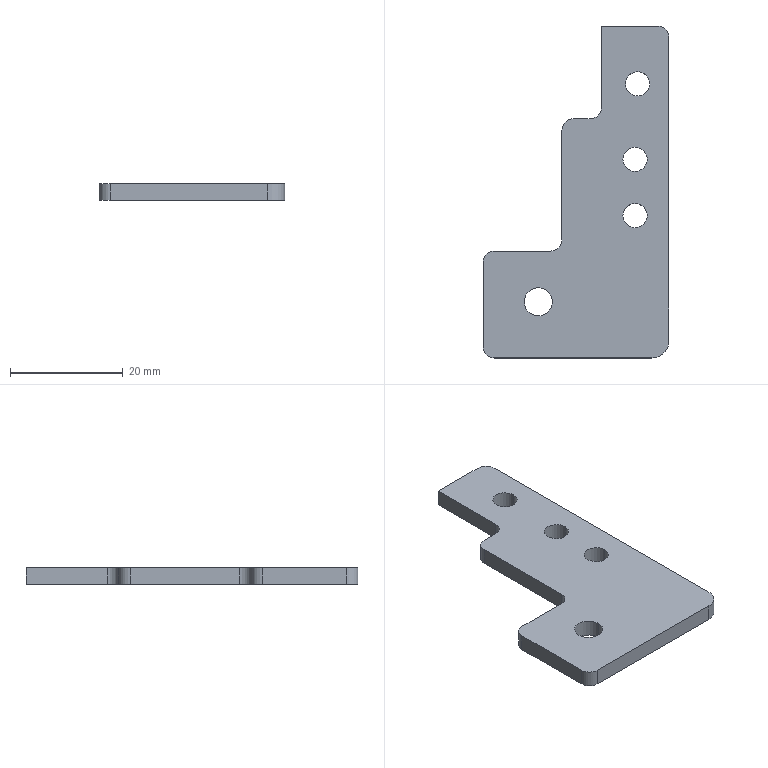Part | SolidWorks | features Cut 4, ICE 4, Fillet 3, MoveFace 2, Extrusion 1, HoleWzd 1 | 1 solid | 25 faces | box 33 x 59 x 3 mm | volume 3614 mm3 | cylinder 15 | plane 10 | commonest cylinder face diameters 4 x6 4.3 x6 5 x2 6 x1
STEP:
#1=CARTESIAN_POINT('',(8.8,19.2,3.));
#2=VERTEX_POINT('',#1);
#3=CARTESIAN_POINT('',(13.1,19.2,3.));
#4=VERTEX_POINT('',#3);
#5=CARTESIAN_POINT('',(10.95,19.2,3.));
#6=DIRECTION('',(0.,0.,1.));
#7=DIRECTION('',(1.,0.,0.));
#8=AXIS2_PLACEMENT_3D('',#5,#6,#7);
#9=CIRCLE('',#8,2.15);
#10=EDGE_CURVE('',#2,#4,#9,.T.);
#11=ORIENTED_EDGE('',*,*,#10,.T.);
#12=CARTESIAN_POINT('',(13.1,19.2,0.));
#13=VERTEX_POINT('',#12);
#14=CARTESIAN_POINT('',(13.1,19.2,0.));
#15=DIRECTION('',(0.,0.,-1.));
#16=VECTOR('',#15,1000.);
#17=LINE('',#14,#16);
#18=EDGE_CURVE('',#4,#13,#17,.T.);
#19=ORIENTED_EDGE('',*,*,#18,.T.);
#20=CARTESIAN_POINT('',(8.8,19.2,0.));
#21=VERTEX_POINT('',#20);
#22=CARTESIAN_POINT('',(10.95,19.2,0.));
#23=DIRECTION('',(0.,0.,-1.));
#24=DIRECTION('',(-1.,0.,0.));
#25=AXIS2_PLACEMENT_3D('',#22,#23,#24);
#26=CIRCLE('',#25,2.15);
#27=EDGE_CURVE('',#13,#21,#26,.T.);
#28=ORIENTED_EDGE('',*,*,#27,.T.);
#29=CARTESIAN_POINT('',(8.8,19.2,0.));
#30=DIRECTION('',(0.,0.,-1.));
#31=VECTOR('',#30,1000.);
#32=LINE('',#29,#31);
#33=EDGE_CURVE('',#2,#21,#32,.T.);
#34=ORIENTED_EDGE('',*,*,#33,.F.);
#35=EDGE_LOOP('',(#11,#19,#28,#34));
#36=FACE_OUTER_BOUND('',#35,.T.);
#37=CARTESIAN_POINT('',(10.95,19.2,0.));
#38=DIRECTION('',(0.,0.,-1.));
#39=DIRECTION('',(-1.,0.,0.));
#40=AXIS2_PLACEMENT_3D('',#37,#38,#39);
#41=CYLINDRICAL_SURFACE('',#40,2.15);
#42=ADVANCED_FACE('',(#36),#41,.F.);
#43=CARTESIAN_POINT('',(-9.2,-19.5,3.));
#44=VERTEX_POINT('',#43);
#45=CARTESIAN_POINT('',(-4.2,-19.5,3.));
#46=VERTEX_POINT('',#45);
#47=CARTESIAN_POINT('',(-6.7,-19.5,3.));
#48=DIRECTION('',(0.,0.,1.));
#49=DIRECTION('',(1.,0.,0.));
#50=AXIS2_PLACEMENT_3D('',#47,#48,#49);
#51=CIRCLE('',#50,2.5);
#52=EDGE_CURVE('',#44,#46,#51,.T.);
#53=ORIENTED_EDGE('',*,*,#52,.T.);
#54=CARTESIAN_POINT('',(-4.2,-19.5,0.));
#55=VERTEX_POINT('',#54);
#56=CARTESIAN_POINT('',(-4.2,-19.5,10.));
#57=DIRECTION('',(0.,0.,-1.));
#58=VECTOR('',#57,1000.);
#59=LINE('',#56,#58);
#60=EDGE_CURVE('',#46,#55,#59,.T.);
#61=ORIENTED_EDGE('',*,*,#60,.T.);
#62=CARTESIAN_POINT('',(-9.2,-19.5,0.));
#63=VERTEX_POINT('',#62);
#64=CARTESIAN_POINT('',(-6.7,-19.5,0.));
#65=DIRECTION('',(0.,0.,-1.));
#66=DIRECTION('',(-1.,0.,0.));
#67=AXIS2_PLACEMENT_3D('',#64,#65,#66);
#68=CIRCLE('',#67,2.5);
#69=EDGE_CURVE('',#55,#63,#68,.T.);
#70=ORIENTED_EDGE('',*,*,#69,.T.);
#71=CARTESIAN_POINT('',(-9.2,-19.5,10.));
#72=DIRECTION('',(0.,0.,-1.));
#73=VECTOR('',#72,1000.);
#74=LINE('',#71,#73);
#75=EDGE_CURVE('',#44,#63,#74,.T.);
#76=ORIENTED_EDGE('',*,*,#75,.F.);
#77=EDGE_LOOP('',(#53,#61,#70,#76));
#78=FACE_OUTER_BOUND('',#77,.T.);
#79=CARTESIAN_POINT('',(-6.7,-19.5,10.));
#80=DIRECTION('',(0.,0.,-1.));
#81=DIRECTION('',(-1.,0.,0.));
#82=AXIS2_PLACEMENT_3D('',#79,#80,#81);
#83=CYLINDRICAL_SURFACE('',#82,2.5);
#84=ADVANCED_FACE('',(#78),#83,.F.);
#85=CARTESIAN_POINT('',(8.35,5.8,3.));
#86=VERTEX_POINT('',#85);
#87=CARTESIAN_POINT('',(12.65,5.8,3.));
#88=VERTEX_POINT('',#87);
#89=CARTESIAN_POINT('',(10.5,5.8,3.));
#90=DIRECTION('',(0.,0.,1.));
#91=DIRECTION('',(1.,0.,0.));
#92=AXIS2_PLACEMENT_3D('',#89,#90,#91);
#93=CIRCLE('',#92,2.15);
#94=EDGE_CURVE('',#86,#88,#93,.T.);
#95=ORIENTED_EDGE('',*,*,#94,.T.);
#96=CARTESIAN_POINT('',(12.65,5.8,0.));
#97=VERTEX_POINT('',#96);
#98=CARTESIAN_POINT('',(12.65,5.8,21.));
#99=DIRECTION('',(0.,0.,-1.));
#100=VECTOR('',#99,1000.);
#101=LINE('',#98,#100);
#102=EDGE_CURVE('',#88,#97,#101,.T.);
#103=ORIENTED_EDGE('',*,*,#102,.T.);
#104=CARTESIAN_POINT('',(8.35,5.8,0.));
#105=VERTEX_POINT('',#104);
#106=CARTESIAN_POINT('',(10.5,5.8,0.));
#107=DIRECTION('',(0.,0.,-1.));
#108=DIRECTION('',(-1.,0.,0.));
#109=AXIS2_PLACEMENT_3D('',#106,#107,#108);
#110=CIRCLE('',#109,2.15);
#111=EDGE_CURVE('',#97,#105,#110,.T.);
#112=ORIENTED_EDGE('',*,*,#111,.T.);
#113=CARTESIAN_POINT('',(8.35,5.8,21.));
#114=DIRECTION('',(0.,0.,-1.));
#115=VECTOR('',#114,1000.);
#116=LINE('',#113,#115);
#117=EDGE_CURVE('',#86,#105,#116,.T.);
#118=ORIENTED_EDGE('',*,*,#117,.F.);
#119=EDGE_LOOP('',(#95,#103,#112,#118));
#120=FACE_OUTER_BOUND('',#119,.T.);
#121=CARTESIAN_POINT('',(10.5,5.8,21.));
#122=DIRECTION('',(0.,0.,-1.));
#123=DIRECTION('',(-1.,0.,0.));
#124=AXIS2_PLACEMENT_3D('',#121,#122,#123);
#125=CYLINDRICAL_SURFACE('',#124,2.15);
#126=ADVANCED_FACE('',(#120),#125,.F.);
#127=CARTESIAN_POINT('',(8.35,-4.2,3.));
#128=VERTEX_POINT('',#127);
#129=CARTESIAN_POINT('',(12.65,-4.2,3.));
#130=VERTEX_POINT('',#129);
#131=CARTESIAN_POINT('',(10.5,-4.2,3.));
#132=DIRECTION('',(0.,0.,1.));
#133=DIRECTION('',(1.,0.,0.));
#134=AXIS2_PLACEMENT_3D('',#131,#132,#133);
#135=CIRCLE('',#134,2.15);
#136=EDGE_CURVE('',#128,#130,#135,.T.);
#137=ORIENTED_EDGE('',*,*,#136,.T.);
#138=CARTESIAN_POINT('',(12.65,-4.2,0.));
#139=VERTEX_POINT('',#138);
#140=CARTESIAN_POINT('',(12.65,-4.2,21.));
#141=DIRECTION('',(0.,0.,-1.));
#142=VECTOR('',#141,1000.);
#143=LINE('',#140,#142);
#144=EDGE_CURVE('',#130,#139,#143,.T.);
#145=ORIENTED_EDGE('',*,*,#144,.T.);
#146=CARTESIAN_POINT('',(8.35,-4.2,0.));
#147=VERTEX_POINT('',#146);
#148=CARTESIAN_POINT('',(10.5,-4.2,0.));
#149=DIRECTION('',(0.,0.,-1.));
#150=DIRECTION('',(-1.,0.,0.));
#151=AXIS2_PLACEMENT_3D('',#148,#149,#150);
#152=CIRCLE('',#151,2.15);
#153=EDGE_CURVE('',#139,#147,#152,.T.);
#154=ORIENTED_EDGE('',*,*,#153,.T.);
#155=CARTESIAN_POINT('',(8.35,-4.2,21.));
#156=DIRECTION('',(0.,0.,-1.));
#157=VECTOR('',#156,1000.);
#158=LINE('',#155,#157);
#159=EDGE_CURVE('',#128,#147,#158,.T.);
#160=ORIENTED_EDGE('',*,*,#159,.F.);
#161=EDGE_LOOP('',(#137,#145,#154,#160));
#162=FACE_OUTER_BOUND('',#161,.T.);
#163=CARTESIAN_POINT('',(10.5,-4.2,21.));
#164=DIRECTION('',(0.,0.,-1.));
#165=DIRECTION('',(-1.,0.,0.));
#166=AXIS2_PLACEMENT_3D('',#163,#164,#165);
#167=CYLINDRICAL_SURFACE('',#166,2.15);
#168=ADVANCED_FACE('',(#162),#167,.F.);
#169=CARTESIAN_POINT('',(16.5,-26.5,0.));
#170=VERTEX_POINT('',#169);
#171=CARTESIAN_POINT('',(16.5,27.5,0.));
#172=VERTEX_POINT('',#171);
#173=CARTESIAN_POINT('',(16.5,29.5,0.));
#174=DIRECTION('',(0.,1.,0.));
#175=VECTOR('',#174,1000.);
#176=LINE('',#173,#175);
#177=EDGE_CURVE('',#170,#172,#176,.T.);
#178=ORIENTED_EDGE('',*,*,#177,.T.);
#179=CARTESIAN_POINT('',(16.5,27.5,3.));
#180=VERTEX_POINT('',#179);
#181=CARTESIAN_POINT('',(16.5,27.5,3.));
#182=DIRECTION('',(0.,0.,1.));
#183=VECTOR('',#182,1000.);
#184=LINE('',#181,#183);
#185=EDGE_CURVE('',#172,#180,#184,.T.);
#186=ORIENTED_EDGE('',*,*,#185,.T.);
#187=CARTESIAN_POINT('',(16.5,-26.5,3.));
#188=VERTEX_POINT('',#187);
#189=CARTESIAN_POINT('',(16.5,29.5,3.));
#190=DIRECTION('',(0.,1.,0.));
#191=VECTOR('',#190,1000.);
#192=LINE('',#189,#191);
#193=EDGE_CURVE('',#188,#180,#192,.T.);
#194=ORIENTED_EDGE('',*,*,#193,.F.);
#195=CARTESIAN_POINT('',(16.5,-26.5,3.));
#196=DIRECTION('',(0.,0.,-1.));
#197=VECTOR('',#196,1000.);
#198=LINE('',#195,#197);
#199=EDGE_CURVE('',#188,#170,#198,.T.);
#200=ORIENTED_EDGE('',*,*,#199,.T.);
#201=EDGE_LOOP('',(#178,#186,#194,#200));
#202=FACE_OUTER_BOUND('',#201,.T.);
#203=CARTESIAN_POINT('',(16.5,29.5,3.));
#204=DIRECTION('',(-1.,0.,0.));
#205=DIRECTION('',(0.,-1.,0.));
#206=AXIS2_PLACEMENT_3D('',#203,#204,#205);
#207=PLANE('',#206);
#208=ADVANCED_FACE('',(#202),#207,.F.);
#209=CARTESIAN_POINT('',(14.5,29.5,0.));
#210=VERTEX_POINT('',#209);
#211=CARTESIAN_POINT('',(4.5,29.5,0.));
#212=VERTEX_POINT('',#211);
#213=CARTESIAN_POINT('',(-16.5,29.5,0.));
#214=DIRECTION('',(-1.,0.,0.));
#215=VECTOR('',#214,1000.);
#216=LINE('',#213,#215);
#217=EDGE_CURVE('',#210,#212,#216,.T.);
#218=ORIENTED_EDGE('',*,*,#217,.T.);
#219=CARTESIAN_POINT('',(4.5,29.5,3.));
#220=VERTEX_POINT('',#219);
#221=CARTESIAN_POINT('',(4.5,29.5,3.));
#222=DIRECTION('',(0.,0.,1.));
#223=VECTOR('',#222,1000.);
#224=LINE('',#221,#223);
#225=EDGE_CURVE('',#212,#220,#224,.T.);
#226=ORIENTED_EDGE('',*,*,#225,.T.);
#227=CARTESIAN_POINT('',(14.5,29.5,3.));
#228=VERTEX_POINT('',#227);
#229=CARTESIAN_POINT('',(-16.5,29.5,3.));
#230=DIRECTION('',(-1.,0.,0.));
#231=VECTOR('',#230,1000.);
#232=LINE('',#229,#231);
#233=EDGE_CURVE('',#228,#220,#232,.T.);
#234=ORIENTED_EDGE('',*,*,#233,.F.);
#235=CARTESIAN_POINT('',(14.5,29.5,3.));
#236=DIRECTION('',(0.,0.,-1.));
#237=VECTOR('',#236,1000.);
#238=LINE('',#235,#237);
#239=EDGE_CURVE('',#228,#210,#238,.T.);
#240=ORIENTED_EDGE('',*,*,#239,.T.);
#241=EDGE_LOOP('',(#218,#226,#234,#240));
#242=FACE_OUTER_BOUND('',#241,.T.);
#243=CARTESIAN_POINT('',(-16.5,29.5,3.));
#244=DIRECTION('',(0.,-1.,0.));
#245=DIRECTION('',(0.,0.,-1.));
#246=AXIS2_PLACEMENT_3D('',#243,#244,#245);
#247=PLANE('',#246);
#248=ADVANCED_FACE('',(#242),#247,.F.);
#249=CARTESIAN_POINT('',(-16.5,-12.5,3.));
#250=VERTEX_POINT('',#249);
#251=CARTESIAN_POINT('',(-16.5,-27.5,3.));
#252=VERTEX_POINT('',#251);
#253=CARTESIAN_POINT('',(-16.5,29.5,3.));
#254=DIRECTION('',(0.,-1.,0.));
#255=VECTOR('',#254,1000.);
#256=LINE('',#253,#255);
#257=EDGE_CURVE('',#250,#252,#256,.T.);
#258=ORIENTED_EDGE('',*,*,#257,.F.);
#259=CARTESIAN_POINT('',(-16.5,-12.5,0.));
#260=VERTEX_POINT('',#259);
#261=CARTESIAN_POINT('',(-16.5,-12.5,3.));
#262=DIRECTION('',(0.,0.,-1.));
#263=VECTOR('',#262,1000.);
#264=LINE('',#261,#263);
#265=EDGE_CURVE('',#250,#260,#264,.T.);
#266=ORIENTED_EDGE('',*,*,#265,.T.);
#267=CARTESIAN_POINT('',(-16.5,-27.5,0.));
#268=VERTEX_POINT('',#267);
#269=CARTESIAN_POINT('',(-16.5,29.5,0.));
#270=DIRECTION('',(0.,-1.,0.));
#271=VECTOR('',#270,1000.);
#272=LINE('',#269,#271);
#273=EDGE_CURVE('',#260,#268,#272,.T.);
#274=ORIENTED_EDGE('',*,*,#273,.T.);
#275=CARTESIAN_POINT('',(-16.5,-27.5,3.));
#276=DIRECTION('',(0.,0.,1.));
#277=VECTOR('',#276,1000.);
#278=LINE('',#275,#277);
#279=EDGE_CURVE('',#268,#252,#278,.T.);
#280=ORIENTED_EDGE('',*,*,#279,.T.);
#281=EDGE_LOOP('',(#258,#266,#274,#280));
#282=FACE_OUTER_BOUND('',#281,.T.);
#283=CARTESIAN_POINT('',(-16.5,29.5,3.));
#284=DIRECTION('',(1.,0.,0.));
#285=DIRECTION('',(0.,1.,0.));
#286=AXIS2_PLACEMENT_3D('',#283,#284,#285);
#287=PLANE('',#286);
#288=ADVANCED_FACE('',(#282),#287,.F.);
#289=CARTESIAN_POINT('',(-14.5,-29.5,3.));
#290=VERTEX_POINT('',#289);
#291=CARTESIAN_POINT('',(13.5,-29.5,3.));
#292=VERTEX_POINT('',#291);
#293=CARTESIAN_POINT('',(-16.5,-29.5,3.));
#294=DIRECTION('',(1.,0.,0.));
#295=VECTOR('',#294,1000.);
#296=LINE('',#293,#295);
#297=EDGE_CURVE('',#290,#292,#296,.T.);
#298=ORIENTED_EDGE('',*,*,#297,.F.);
#299=CARTESIAN_POINT('',(-14.5,-29.5,0.));
#300=VERTEX_POINT('',#299);
#301=CARTESIAN_POINT('',(-14.5,-29.5,3.));
#302=DIRECTION('',(0.,0.,-1.));
#303=VECTOR('',#302,1000.);
#304=LINE('',#301,#303);
#305=EDGE_CURVE('',#290,#300,#304,.T.);
#306=ORIENTED_EDGE('',*,*,#305,.T.);
#307=CARTESIAN_POINT('',(13.5,-29.5,0.));
#308=VERTEX_POINT('',#307);
#309=CARTESIAN_POINT('',(-16.5,-29.5,0.));
#310=DIRECTION('',(1.,0.,0.));
#311=VECTOR('',#310,1000.);
#312=LINE('',#309,#311);
#313=EDGE_CURVE('',#300,#308,#312,.T.);
#314=ORIENTED_EDGE('',*,*,#313,.T.);
#315=CARTESIAN_POINT('',(13.5,-29.5,3.));
#316=DIRECTION('',(0.,0.,1.));
#317=VECTOR('',#316,1000.);
#318=LINE('',#315,#317);
#319=EDGE_CURVE('',#308,#292,#318,.T.);
#320=ORIENTED_EDGE('',*,*,#319,.T.);
#321=EDGE_LOOP('',(#298,#306,#314,#320));
#322=FACE_OUTER_BOUND('',#321,.T.);
#323=CARTESIAN_POINT('',(-16.5,-29.5,3.));
#324=DIRECTION('',(0.,1.,0.));
#325=DIRECTION('',(0.,0.,1.));
#326=AXIS2_PLACEMENT_3D('',#323,#324,#325);
#327=PLANE('',#326);
#328=ADVANCED_FACE('',(#322),#327,.F.);
#329=ORIENTED_EDGE('',*,*,#10,.F.);
#330=CARTESIAN_POINT('',(10.95,19.2,3.));
#331=DIRECTION('',(0.,0.,1.));
#332=DIRECTION('',(1.,0.,0.));
#333=AXIS2_PLACEMENT_3D('',#330,#331,#332);
#334=CIRCLE('',#333,2.15);
#335=EDGE_CURVE('',#4,#2,#334,.T.);
#336=ORIENTED_EDGE('',*,*,#335,.F.);
#337=EDGE_LOOP('',(#329,#336));
#338=FACE_BOUND('',#337,.T.);
#339=ORIENTED_EDGE('',*,*,#52,.F.);
#340=CARTESIAN_POINT('',(-6.7,-19.5,3.));
#341=DIRECTION('',(0.,0.,1.));
#342=DIRECTION('',(1.,0.,0.));
#343=AXIS2_PLACEMENT_3D('',#340,#341,#342);
#344=CIRCLE('',#343,2.5);
#345=EDGE_CURVE('',#46,#44,#344,.T.);
#346=ORIENTED_EDGE('',*,*,#345,.F.);
#347=EDGE_LOOP('',(#339,#346));
#348=FACE_BOUND('',#347,.T.);
#349=ORIENTED_EDGE('',*,*,#233,.T.);
#350=CARTESIAN_POINT('',(4.5,15.,3.));
#351=VERTEX_POINT('',#350);
#352=CARTESIAN_POINT('',(4.5,25.,3.));
#353=DIRECTION('',(0.,-1.,0.));
#354=VECTOR('',#353,1000.);
#355=LINE('',#352,#354);
#356=EDGE_CURVE('',#220,#351,#355,.T.);
#357=ORIENTED_EDGE('',*,*,#356,.T.);
#358=CARTESIAN_POINT('',(2.5,13.,3.));
#359=VERTEX_POINT('',#358);
#360=CARTESIAN_POINT('',(2.5,15.,3.));
#361=DIRECTION('',(0.,0.,-1.));
#362=DIRECTION('',(1.,0.,0.));
#363=AXIS2_PLACEMENT_3D('',#360,#361,#362);
#364=CIRCLE('',#363,2.);
#365=EDGE_CURVE('',#351,#359,#364,.T.);
#366=ORIENTED_EDGE('',*,*,#365,.T.);
#367=CARTESIAN_POINT('',(-0.5,13.,3.));
#368=VERTEX_POINT('',#367);
#369=CARTESIAN_POINT('',(4.5,13.,3.));
#370=DIRECTION('',(-1.,0.,0.));
#371=VECTOR('',#370,1000.);
#372=LINE('',#369,#371);
#373=EDGE_CURVE('',#359,#368,#372,.T.);
#374=ORIENTED_EDGE('',*,*,#373,.T.);
#375=CARTESIAN_POINT('',(-2.5,11.,3.));
#376=VERTEX_POINT('',#375);
#377=CARTESIAN_POINT('',(-0.5,11.,3.));
#378=DIRECTION('',(0.,0.,1.));
#379=DIRECTION('',(1.,0.,0.));
#380=AXIS2_PLACEMENT_3D('',#377,#378,#379);
#381=CIRCLE('',#380,2.);
#382=EDGE_CURVE('',#368,#376,#381,.T.);
#383=ORIENTED_EDGE('',*,*,#382,.T.);
#384=CARTESIAN_POINT('',(-2.5,-8.5,3.));
#385=VERTEX_POINT('',#384);
#386=CARTESIAN_POINT('',(-2.5,29.5,3.));
#387=DIRECTION('',(0.,-1.,0.));
#388=VECTOR('',#387,1000.);
#389=LINE('',#386,#388);
#390=EDGE_CURVE('',#376,#385,#389,.T.);
#391=ORIENTED_EDGE('',*,*,#390,.T.);
#392=CARTESIAN_POINT('',(-4.5,-10.5,3.));
#393=VERTEX_POINT('',#392);
#394=CARTESIAN_POINT('',(-4.5,-8.5,3.));
#395=DIRECTION('',(0.,0.,-1.));
#396=DIRECTION('',(1.,0.,0.));
#397=AXIS2_PLACEMENT_3D('',#394,#395,#396);
#398=CIRCLE('',#397,2.);
#399=EDGE_CURVE('',#385,#393,#398,.T.);
#400=ORIENTED_EDGE('',*,*,#399,.T.);
#401=CARTESIAN_POINT('',(-14.5,-10.5,3.));
#402=VERTEX_POINT('',#401);
#403=CARTESIAN_POINT('',(-16.5,-10.5,3.));
#404=DIRECTION('',(-1.,0.,0.));
#405=VECTOR('',#404,1000.);
#406=LINE('',#403,#405);
#407=EDGE_CURVE('',#393,#402,#406,.T.);
#408=ORIENTED_EDGE('',*,*,#407,.T.);
#409=CARTESIAN_POINT('',(-14.5,-12.5,3.));
#410=DIRECTION('',(0.,0.,1.));
#411=DIRECTION('',(1.,0.,0.));
#412=AXIS2_PLACEMENT_3D('',#409,#410,#411);
#413=CIRCLE('',#412,2.);
#414=EDGE_CURVE('',#402,#250,#413,.T.);
#415=ORIENTED_EDGE('',*,*,#414,.T.);
#416=ORIENTED_EDGE('',*,*,#257,.T.);
#417=CARTESIAN_POINT('',(-14.5,-27.5,3.));
#418=DIRECTION('',(0.,0.,1.));
#419=DIRECTION('',(1.,0.,0.));
#420=AXIS2_PLACEMENT_3D('',#417,#418,#419);
#421=CIRCLE('',#420,2.);
#422=EDGE_CURVE('',#252,#290,#421,.T.);
#423=ORIENTED_EDGE('',*,*,#422,.T.);
#424=ORIENTED_EDGE('',*,*,#297,.T.);
#425=CARTESIAN_POINT('',(13.5,-26.5,3.));
#426=DIRECTION('',(0.,0.,1.));
#427=DIRECTION('',(1.,0.,0.));
#428=AXIS2_PLACEMENT_3D('',#425,#426,#427);
#429=CIRCLE('',#428,3.);
#430=EDGE_CURVE('',#292,#188,#429,.T.);
#431=ORIENTED_EDGE('',*,*,#430,.T.);
#432=ORIENTED_EDGE('',*,*,#193,.T.);
#433=CARTESIAN_POINT('',(14.5,27.5,3.));
#434=DIRECTION('',(0.,0.,1.));
#435=DIRECTION('',(1.,0.,0.));
#436=AXIS2_PLACEMENT_3D('',#433,#434,#435);
#437=CIRCLE('',#436,2.);
#438=EDGE_CURVE('',#180,#228,#437,.T.);
#439=ORIENTED_EDGE('',*,*,#438,.T.);
#440=EDGE_LOOP('',(#349,#357,#366,#374,#383,#391,#400,#408,#415,#416,#423,#424,#431,#432,#439));
#441=FACE_OUTER_BOUND('',#440,.T.);
#442=ORIENTED_EDGE('',*,*,#94,.F.);
#443=CARTESIAN_POINT('',(10.5,5.8,3.));
#444=DIRECTION('',(0.,0.,1.));
#445=DIRECTION('',(1.,0.,0.));
#446=AXIS2_PLACEMENT_3D('',#443,#444,#445);
#447=CIRCLE('',#446,2.15);
#448=EDGE_CURVE('',#88,#86,#447,.T.);
#449=ORIENTED_EDGE('',*,*,#448,.F.);
#450=EDGE_LOOP('',(#442,#449));
#451=FACE_BOUND('',#450,.T.);
#452=ORIENTED_EDGE('',*,*,#136,.F.);
#453=CARTESIAN_POINT('',(10.5,-4.2,3.));
#454=DIRECTION('',(0.,0.,1.));
#455=DIRECTION('',(1.,0.,0.));
#456=AXIS2_PLACEMENT_3D('',#453,#454,#455);
#457=CIRCLE('',#456,2.15);
#458=EDGE_CURVE('',#130,#128,#457,.T.);
#459=ORIENTED_EDGE('',*,*,#458,.F.);
#460=EDGE_LOOP('',(#452,#459));
#461=FACE_BOUND('',#460,.T.);
#462=CARTESIAN_POINT('',(0.,0.,3.));
#463=DIRECTION('',(0.,0.,1.));
#464=DIRECTION('',(1.,0.,0.));
#465=AXIS2_PLACEMENT_3D('',#462,#463,#464);
#466=PLANE('',#465);
#467=ADVANCED_FACE('',(#338,#348,#441,#451,#461),#466,.T.);
#468=CARTESIAN_POINT('',(10.95,19.2,0.));
#469=DIRECTION('',(0.,0.,-1.));
#470=DIRECTION('',(-1.,0.,0.));
#471=AXIS2_PLACEMENT_3D('',#468,#469,#470);
#472=CIRCLE('',#471,2.15);
#473=EDGE_CURVE('',#21,#13,#472,.T.);
#474=ORIENTED_EDGE('',*,*,#473,.F.);
#475=ORIENTED_EDGE('',*,*,#27,.F.);
#476=EDGE_LOOP('',(#474,#475));
#477=FACE_BOUND('',#476,.T.);
#478=CARTESIAN_POINT('',(-6.7,-19.5,0.));
#479=DIRECTION('',(0.,0.,-1.));
#480=DIRECTION('',(-1.,0.,0.));
#481=AXIS2_PLACEMENT_3D('',#478,#479,#480);
#482=CIRCLE('',#481,2.5);
#483=EDGE_CURVE('',#63,#55,#482,.T.);
#484=ORIENTED_EDGE('',*,*,#483,.F.);
#485=ORIENTED_EDGE('',*,*,#69,.F.);
#486=EDGE_LOOP('',(#484,#485));
#487=FACE_BOUND('',#486,.T.);
#488=CARTESIAN_POINT('',(10.5,5.8,0.));
#489=DIRECTION('',(0.,0.,-1.));
#490=DIRECTION('',(-1.,0.,0.));
#491=AXIS2_PLACEMENT_3D('',#488,#489,#490);
#492=CIRCLE('',#491,2.15);
#493=EDGE_CURVE('',#105,#97,#492,.T.);
#494=ORIENTED_EDGE('',*,*,#493,.F.);
#495=ORIENTED_EDGE('',*,*,#111,.F.);
#496=EDGE_LOOP('',(#494,#495));
#497=FACE_BOUND('',#496,.T.);
#498=CARTESIAN_POINT('',(10.5,-4.2,0.));
#499=DIRECTION('',(0.,0.,-1.));
#500=DIRECTION('',(-1.,0.,0.));
#501=AXIS2_PLACEMENT_3D('',#498,#499,#500);
#502=CIRCLE('',#501,2.15);
#503=EDGE_CURVE('',#147,#139,#502,.T.);
#504=ORIENTED_EDGE('',*,*,#503,.F.);
#505=ORIENTED_EDGE('',*,*,#153,.F.);
#506=EDGE_LOOP('',(#504,#505));
#507=FACE_BOUND('',#506,.T.);
#508=CARTESIAN_POINT('',(4.5,15.,0.));
#509=VERTEX_POINT('',#508);
#510=CARTESIAN_POINT('',(4.5,25.,0.));
#511=DIRECTION('',(0.,-1.,0.));
#512=VECTOR('',#511,1000.);
#513=LINE('',#510,#512);
#514=EDGE_CURVE('',#212,#509,#513,.T.);
#515=ORIENTED_EDGE('',*,*,#514,.F.);
#516=ORIENTED_EDGE('',*,*,#217,.F.);
#517=CARTESIAN_POINT('',(14.5,27.5,0.));
#518=DIRECTION('',(0.,0.,-1.));
#519=DIRECTION('',(1.,0.,0.));
#520=AXIS2_PLACEMENT_3D('',#517,#518,#519);
#521=CIRCLE('',#520,2.);
#522=EDGE_CURVE('',#210,#172,#521,.T.);
#523=ORIENTED_EDGE('',*,*,#522,.T.);
#524=ORIENTED_EDGE('',*,*,#177,.F.);
#525=CARTESIAN_POINT('',(13.5,-26.5,0.));
#526=DIRECTION('',(0.,0.,-1.));
#527=DIRECTION('',(1.,0.,0.));
#528=AXIS2_PLACEMENT_3D('',#525,#526,#527);
#529=CIRCLE('',#528,3.);
#530=EDGE_CURVE('',#170,#308,#529,.T.);
#531=ORIENTED_EDGE('',*,*,#530,.T.);
#532=ORIENTED_EDGE('',*,*,#313,.F.);
#533=CARTESIAN_POINT('',(-14.5,-27.5,0.));
#534=DIRECTION('',(0.,0.,-1.));
#535=DIRECTION('',(1.,0.,0.));
#536=AXIS2_PLACEMENT_3D('',#533,#534,#535);
#537=CIRCLE('',#536,2.);
#538=EDGE_CURVE('',#300,#268,#537,.T.);
#539=ORIENTED_EDGE('',*,*,#538,.T.);
#540=ORIENTED_EDGE('',*,*,#273,.F.);
#541=CARTESIAN_POINT('',(-14.5,-10.5,0.));
#542=VERTEX_POINT('',#541);
#543=CARTESIAN_POINT('',(-14.5,-12.5,0.));
#544=DIRECTION('',(0.,0.,-1.));
#545=DIRECTION('',(1.,0.,0.));
#546=AXIS2_PLACEMENT_3D('',#543,#544,#545);
#547=CIRCLE('',#546,2.);
#548=EDGE_CURVE('',#260,#542,#547,.T.);
#549=ORIENTED_EDGE('',*,*,#548,.T.);
#550=CARTESIAN_POINT('',(-4.5,-10.5,0.));
#551=VERTEX_POINT('',#550);
#552=CARTESIAN_POINT('',(-16.5,-10.5,0.));
#553=DIRECTION('',(-1.,0.,0.));
#554=VECTOR('',#553,1000.);
#555=LINE('',#552,#554);
#556=EDGE_CURVE('',#551,#542,#555,.T.);
#557=ORIENTED_EDGE('',*,*,#556,.F.);
#558=CARTESIAN_POINT('',(-2.5,-8.5,0.));
#559=VERTEX_POINT('',#558);
#560=CARTESIAN_POINT('',(-4.5,-8.5,0.));
#561=DIRECTION('',(0.,0.,1.));
#562=DIRECTION('',(1.,0.,0.));
#563=AXIS2_PLACEMENT_3D('',#560,#561,#562);
#564=CIRCLE('',#563,2.);
#565=EDGE_CURVE('',#551,#559,#564,.T.);
#566=ORIENTED_EDGE('',*,*,#565,.T.);
#567=CARTESIAN_POINT('',(-2.5,11.,0.));
#568=VERTEX_POINT('',#567);
#569=CARTESIAN_POINT('',(-2.5,29.5,0.));
#570=DIRECTION('',(0.,-1.,0.));
#571=VECTOR('',#570,1000.);
#572=LINE('',#569,#571);
#573=EDGE_CURVE('',#568,#559,#572,.T.);
#574=ORIENTED_EDGE('',*,*,#573,.F.);
#575=CARTESIAN_POINT('',(-0.5,13.,0.));
#576=VERTEX_POINT('',#575);
#577=CARTESIAN_POINT('',(-0.5,11.,0.));
#578=DIRECTION('',(0.,0.,-1.));
#579=DIRECTION('',(1.,0.,0.));
#580=AXIS2_PLACEMENT_3D('',#577,#578,#579);
#581=CIRCLE('',#580,2.);
#582=EDGE_CURVE('',#568,#576,#581,.T.);
#583=ORIENTED_EDGE('',*,*,#582,.T.);
#584=CARTESIAN_POINT('',(2.5,13.,0.));
#585=VERTEX_POINT('',#584);
#586=CARTESIAN_POINT('',(4.5,13.,0.));
#587=DIRECTION('',(-1.,0.,0.));
#588=VECTOR('',#587,1000.);
#589=LINE('',#586,#588);
#590=EDGE_CURVE('',#585,#576,#589,.T.);
#591=ORIENTED_EDGE('',*,*,#590,.F.);
#592=CARTESIAN_POINT('',(2.5,15.,0.));
#593=DIRECTION('',(0.,0.,1.));
#594=DIRECTION('',(1.,0.,0.));
#595=AXIS2_PLACEMENT_3D('',#592,#593,#594);
#596=CIRCLE('',#595,2.);
#597=EDGE_CURVE('',#585,#509,#596,.T.);
#598=ORIENTED_EDGE('',*,*,#597,.T.);
#599=EDGE_LOOP('',(#515,#516,#523,#524,#531,#532,#539,#540,#549,#557,#566,#574,#583,#591,#598));
#600=FACE_OUTER_BOUND('',#599,.T.);
#601=CARTESIAN_POINT('',(0.,0.,0.));
#602=DIRECTION('',(0.,0.,1.));
#603=DIRECTION('',(1.,0.,0.));
#604=AXIS2_PLACEMENT_3D('',#601,#602,#603);
#605=PLANE('',#604);
#606=ADVANCED_FACE('',(#477,#487,#497,#507,#600),#605,.F.);
#607=ORIENTED_EDGE('',*,*,#556,.T.);
#608=CARTESIAN_POINT('',(-14.5,-10.5,3.));
#609=DIRECTION('',(0.,0.,1.));
#610=VECTOR('',#609,1000.);
#611=LINE('',#608,#610);
#612=EDGE_CURVE('',#542,#402,#611,.T.);
#613=ORIENTED_EDGE('',*,*,#612,.T.);
#614=ORIENTED_EDGE('',*,*,#407,.F.);
#615=CARTESIAN_POINT('',(-4.5,-10.5,0.));
#616=DIRECTION('',(0.,0.,-1.));
#617=VECTOR('',#616,1000.);
#618=LINE('',#615,#617);
#619=EDGE_CURVE('',#393,#551,#618,.T.);
#620=ORIENTED_EDGE('',*,*,#619,.T.);
#621=EDGE_LOOP('',(#607,#613,#614,#620));
#622=FACE_OUTER_BOUND('',#621,.T.);
#623=CARTESIAN_POINT('',(-16.5,-10.5,3.));
#624=DIRECTION('',(0.,-1.,0.));
#625=DIRECTION('',(1.,0.,0.));
#626=AXIS2_PLACEMENT_3D('',#623,#624,#625);
#627=PLANE('',#626);
#628=ADVANCED_FACE('',(#622),#627,.F.);
#629=ORIENTED_EDGE('',*,*,#390,.F.);
#630=CARTESIAN_POINT('',(-2.5,11.,3.));
#631=DIRECTION('',(0.,0.,-1.));
#632=VECTOR('',#631,1000.);
#633=LINE('',#630,#632);
#634=EDGE_CURVE('',#376,#568,#633,.T.);
#635=ORIENTED_EDGE('',*,*,#634,.T.);
#636=ORIENTED_EDGE('',*,*,#573,.T.);
#637=CARTESIAN_POINT('',(-2.5,-8.5,3.));
#638=DIRECTION('',(0.,0.,1.));
#639=VECTOR('',#638,1000.);
#640=LINE('',#637,#639);
#641=EDGE_CURVE('',#559,#385,#640,.T.);
#642=ORIENTED_EDGE('',*,*,#641,.T.);
#643=EDGE_LOOP('',(#629,#635,#636,#642));
#644=FACE_OUTER_BOUND('',#643,.T.);
#645=CARTESIAN_POINT('',(-2.5,29.5,3.));
#646=DIRECTION('',(1.,0.,0.));
#647=DIRECTION('',(0.,1.,0.));
#648=AXIS2_PLACEMENT_3D('',#645,#646,#647);
#649=PLANE('',#648);
#650=ADVANCED_FACE('',(#644),#649,.F.);
#651=ORIENTED_EDGE('',*,*,#430,.F.);
#652=ORIENTED_EDGE('',*,*,#319,.F.);
#653=ORIENTED_EDGE('',*,*,#530,.F.);
#654=ORIENTED_EDGE('',*,*,#199,.F.);
#655=EDGE_LOOP('',(#651,#652,#653,#654));
#656=FACE_OUTER_BOUND('',#655,.T.);
#657=CARTESIAN_POINT('',(13.5,-26.5,3.));
#658=DIRECTION('',(0.,0.,-1.));
#659=DIRECTION('',(-1.,0.,0.));
#660=AXIS2_PLACEMENT_3D('',#657,#658,#659);
#661=CYLINDRICAL_SURFACE('',#660,3.);
#662=ADVANCED_FACE('',(#656),#661,.T.);
#663=ORIENTED_EDGE('',*,*,#590,.T.);
#664=CARTESIAN_POINT('',(-0.5,13.,3.));
#665=DIRECTION('',(0.,0.,1.));
#666=VECTOR('',#665,1000.);
#667=LINE('',#664,#666);
#668=EDGE_CURVE('',#576,#368,#667,.T.);
#669=ORIENTED_EDGE('',*,*,#668,.T.);
#670=ORIENTED_EDGE('',*,*,#373,.F.);
#671=CARTESIAN_POINT('',(2.5,13.,0.));
#672=DIRECTION('',(0.,0.,-1.));
#673=VECTOR('',#672,1000.);
#674=LINE('',#671,#673);
#675=EDGE_CURVE('',#359,#585,#674,.T.);
#676=ORIENTED_EDGE('',*,*,#675,.T.);
#677=EDGE_LOOP('',(#663,#669,#670,#676));
#678=FACE_OUTER_BOUND('',#677,.T.);
#679=CARTESIAN_POINT('',(4.5,13.,3.));
#680=DIRECTION('',(0.,-1.,0.));
#681=DIRECTION('',(0.,0.,-1.));
#682=AXIS2_PLACEMENT_3D('',#679,#680,#681);
#683=PLANE('',#682);
#684=ADVANCED_FACE('',(#678),#683,.F.);
#685=CARTESIAN_POINT('',(4.5,15.,3.));
#686=DIRECTION('',(0.,0.,1.));
#687=VECTOR('',#686,1000.);
#688=LINE('',#685,#687);
#689=EDGE_CURVE('',#509,#351,#688,.T.);
#690=ORIENTED_EDGE('',*,*,#689,.T.);
#691=ORIENTED_EDGE('',*,*,#356,.F.);
#692=ORIENTED_EDGE('',*,*,#225,.F.);
#693=ORIENTED_EDGE('',*,*,#514,.T.);
#694=EDGE_LOOP('',(#690,#691,#692,#693));
#695=FACE_OUTER_BOUND('',#694,.T.);
#696=CARTESIAN_POINT('',(4.5,25.,3.));
#697=DIRECTION('',(1.,0.,0.));
#698=DIRECTION('',(0.,1.,0.));
#699=AXIS2_PLACEMENT_3D('',#696,#697,#698);
#700=PLANE('',#699);
#701=ADVANCED_FACE('',(#695),#700,.F.);
#702=ORIENTED_EDGE('',*,*,#365,.F.);
#703=ORIENTED_EDGE('',*,*,#689,.F.);
#704=ORIENTED_EDGE('',*,*,#597,.F.);
#705=ORIENTED_EDGE('',*,*,#675,.F.);
#706=EDGE_LOOP('',(#702,#703,#704,#705));
#707=FACE_OUTER_BOUND('',#706,.T.);
#708=CARTESIAN_POINT('',(2.5,15.,3.));
#709=DIRECTION('',(0.,0.,1.));
#710=DIRECTION('',(1.,0.,0.));
#711=AXIS2_PLACEMENT_3D('',#708,#709,#710);
#712=CYLINDRICAL_SURFACE('',#711,2.);
#713=ADVANCED_FACE('',(#707),#712,.F.);
#714=ORIENTED_EDGE('',*,*,#414,.F.);
#715=ORIENTED_EDGE('',*,*,#612,.F.);
#716=ORIENTED_EDGE('',*,*,#548,.F.);
#717=ORIENTED_EDGE('',*,*,#265,.F.);
#718=EDGE_LOOP('',(#714,#715,#716,#717));
#719=FACE_OUTER_BOUND('',#718,.T.);
#720=CARTESIAN_POINT('',(-14.5,-12.5,3.));
#721=DIRECTION('',(0.,0.,-1.));
#722=DIRECTION('',(-1.,0.,0.));
#723=AXIS2_PLACEMENT_3D('',#720,#721,#722);
#724=CYLINDRICAL_SURFACE('',#723,2.);
#725=ADVANCED_FACE('',(#719),#724,.T.);
#726=ORIENTED_EDGE('',*,*,#382,.F.);
#727=ORIENTED_EDGE('',*,*,#668,.F.);
#728=ORIENTED_EDGE('',*,*,#582,.F.);
#729=ORIENTED_EDGE('',*,*,#634,.F.);
#730=EDGE_LOOP('',(#726,#727,#728,#729));
#731=FACE_OUTER_BOUND('',#730,.T.);
#732=CARTESIAN_POINT('',(-0.5,11.,3.));
#733=DIRECTION('',(0.,0.,-1.));
#734=DIRECTION('',(-1.,0.,0.));
#735=AXIS2_PLACEMENT_3D('',#732,#733,#734);
#736=CYLINDRICAL_SURFACE('',#735,2.);
#737=ADVANCED_FACE('',(#731),#736,.T.);
#738=ORIENTED_EDGE('',*,*,#399,.F.);
#739=ORIENTED_EDGE('',*,*,#641,.F.);
#740=ORIENTED_EDGE('',*,*,#565,.F.);
#741=ORIENTED_EDGE('',*,*,#619,.F.);
#742=EDGE_LOOP('',(#738,#739,#740,#741));
#743=FACE_OUTER_BOUND('',#742,.T.);
#744=CARTESIAN_POINT('',(-4.5,-8.5,3.));
#745=DIRECTION('',(0.,0.,1.));
#746=DIRECTION('',(1.,0.,0.));
#747=AXIS2_PLACEMENT_3D('',#744,#745,#746);
#748=CYLINDRICAL_SURFACE('',#747,2.);
#749=ADVANCED_FACE('',(#743),#748,.F.);
#750=ORIENTED_EDGE('',*,*,#438,.F.);
#751=ORIENTED_EDGE('',*,*,#185,.F.);
#752=ORIENTED_EDGE('',*,*,#522,.F.);
#753=ORIENTED_EDGE('',*,*,#239,.F.);
#754=EDGE_LOOP('',(#750,#751,#752,#753));
#755=FACE_OUTER_BOUND('',#754,.T.);
#756=CARTESIAN_POINT('',(14.5,27.5,3.));
#757=DIRECTION('',(0.,0.,-1.));
#758=DIRECTION('',(-1.,0.,0.));
#759=AXIS2_PLACEMENT_3D('',#756,#757,#758);
#760=CYLINDRICAL_SURFACE('',#759,2.);
#761=ADVANCED_FACE('',(#755),#760,.T.);
#762=ORIENTED_EDGE('',*,*,#422,.F.);
#763=ORIENTED_EDGE('',*,*,#279,.F.);
#764=ORIENTED_EDGE('',*,*,#538,.F.);
#765=ORIENTED_EDGE('',*,*,#305,.F.);
#766=EDGE_LOOP('',(#762,#763,#764,#765));
#767=FACE_OUTER_BOUND('',#766,.T.);
#768=CARTESIAN_POINT('',(-14.5,-27.5,3.));
#769=DIRECTION('',(0.,0.,-1.));
#770=DIRECTION('',(-1.,0.,0.));
#771=AXIS2_PLACEMENT_3D('',#768,#769,#770);
#772=CYLINDRICAL_SURFACE('',#771,2.);
#773=ADVANCED_FACE('',(#767),#772,.T.);
#774=ORIENTED_EDGE('',*,*,#144,.F.);
#775=ORIENTED_EDGE('',*,*,#458,.T.);
#776=ORIENTED_EDGE('',*,*,#159,.T.);
#777=ORIENTED_EDGE('',*,*,#503,.T.);
#778=EDGE_LOOP('',(#774,#775,#776,#777));
#779=FACE_OUTER_BOUND('',#778,.T.);
#780=CARTESIAN_POINT('',(10.5,-4.2,21.));
#781=DIRECTION('',(0.,0.,-1.));
#782=DIRECTION('',(-1.,0.,0.));
#783=AXIS2_PLACEMENT_3D('',#780,#781,#782);
#784=CYLINDRICAL_SURFACE('',#783,2.15);
#785=ADVANCED_FACE('',(#779),#784,.F.);
#786=ORIENTED_EDGE('',*,*,#102,.F.);
#787=ORIENTED_EDGE('',*,*,#448,.T.);
#788=ORIENTED_EDGE('',*,*,#117,.T.);
#789=ORIENTED_EDGE('',*,*,#493,.T.);
#790=EDGE_LOOP('',(#786,#787,#788,#789));
#791=FACE_OUTER_BOUND('',#790,.T.);
#792=CARTESIAN_POINT('',(10.5,5.8,21.));
#793=DIRECTION('',(0.,0.,-1.));
#794=DIRECTION('',(-1.,0.,0.));
#795=AXIS2_PLACEMENT_3D('',#792,#793,#794);
#796=CYLINDRICAL_SURFACE('',#795,2.15);
#797=ADVANCED_FACE('',(#791),#796,.F.);
#798=ORIENTED_EDGE('',*,*,#60,.F.);
#799=ORIENTED_EDGE('',*,*,#345,.T.);
#800=ORIENTED_EDGE('',*,*,#75,.T.);
#801=ORIENTED_EDGE('',*,*,#483,.T.);
#802=EDGE_LOOP('',(#798,#799,#800,#801));
#803=FACE_OUTER_BOUND('',#802,.T.);
#804=CARTESIAN_POINT('',(-6.7,-19.5,10.));
#805=DIRECTION('',(0.,0.,-1.));
#806=DIRECTION('',(-1.,0.,0.));
#807=AXIS2_PLACEMENT_3D('',#804,#805,#806);
#808=CYLINDRICAL_SURFACE('',#807,2.5);
#809=ADVANCED_FACE('',(#803),#808,.F.);
#810=ORIENTED_EDGE('',*,*,#18,.F.);
#811=ORIENTED_EDGE('',*,*,#335,.T.);
#812=ORIENTED_EDGE('',*,*,#33,.T.);
#813=ORIENTED_EDGE('',*,*,#473,.T.);
#814=EDGE_LOOP('',(#810,#811,#812,#813));
#815=FACE_OUTER_BOUND('',#814,.T.);
#816=CARTESIAN_POINT('',(10.95,19.2,0.));
#817=DIRECTION('',(0.,0.,-1.));
#818=DIRECTION('',(-1.,0.,0.));
#819=AXIS2_PLACEMENT_3D('',#816,#817,#818);
#820=CYLINDRICAL_SURFACE('',#819,2.15);
#821=ADVANCED_FACE('',(#815),#820,.F.);
#822=CLOSED_SHELL('',(#42,#84,#126,#168,#208,#248,#288,#328,#467,#606,#628,#650,#662,#684,#701,#713,#725,#737,#749,#761,#773,#785,#797,#809,#821));
#823=MANIFOLD_SOLID_BREP('',#822);
#824=CARTESIAN_POINT('',(0.,0.,0.));
#825=DIRECTION('',(0.,0.,1.));
#826=DIRECTION('',(1.,0.,0.));
#827=AXIS2_PLACEMENT_3D('',#824,#825,#826);
#828=(LENGTH_UNIT()NAMED_UNIT(*)SI_UNIT(.MILLI.,.METRE.));
#829=UNCERTAINTY_MEASURE_WITH_UNIT(LENGTH_MEASURE(0.00001),#828,'','');
#830=(NAMED_UNIT(*)PLANE_ANGLE_UNIT()SI_UNIT($,.RADIAN.));
#831=(NAMED_UNIT(*)SI_UNIT($,.STERADIAN.)SOLID_ANGLE_UNIT());
#832=(GEOMETRIC_REPRESENTATION_CONTEXT(3)GLOBAL_UNCERTAINTY_ASSIGNED_CONTEXT((#829))GLOBAL_UNIT_ASSIGNED_CONTEXT((#828,#830,#831))REPRESENTATION_CONTEXT('',''));
#833=ADVANCED_BREP_SHAPE_REPRESENTATION('',(#823,#827),#832);